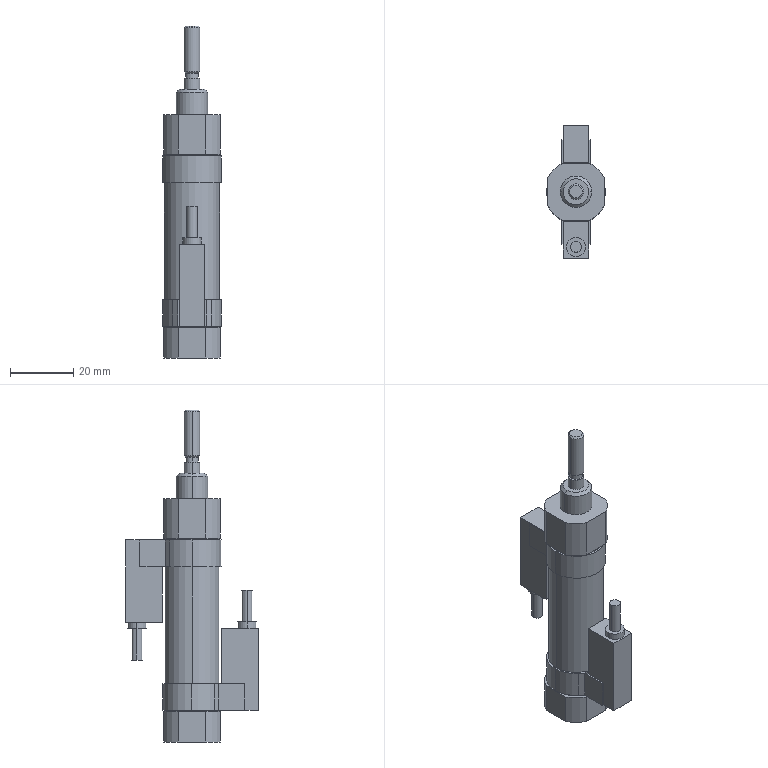Part | STEP file | Bag feed cylinder CDJ2B16-30-C76 (0) | 1 solid | 105 faces | box 18.6 x 41.8 x 105 mm | volume 26186 mm3 | plane 53 | cylinder 42 | cone 10 | commonest cylinder face diameters 18.6 x8 20 x8 17.4 x6 3.4 x4 4.13 x4 5 x4